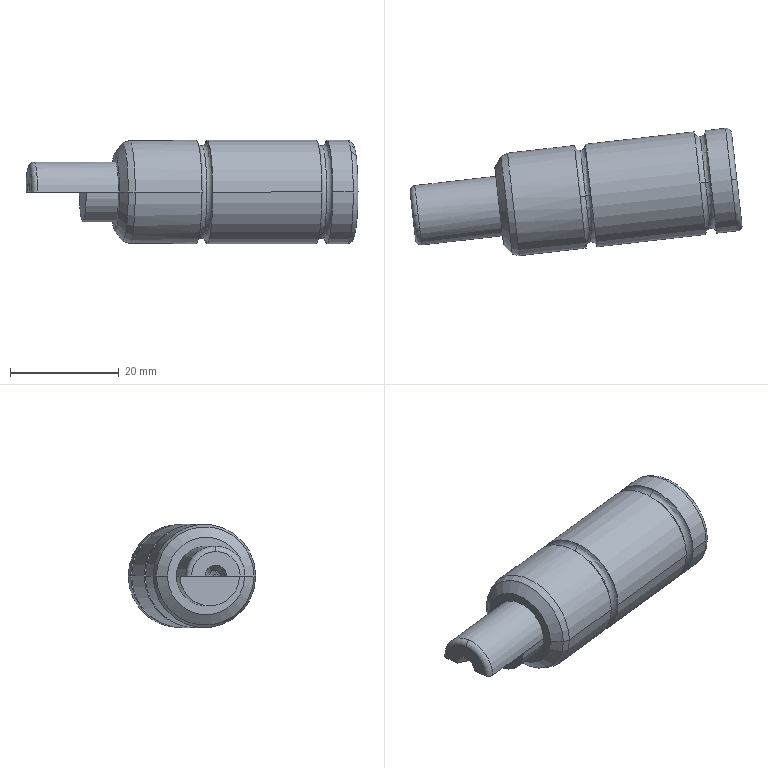Part | NX | features XQ 2 | 1 solid | 174 faces | box 61.099 x 23.455 x 19 mm | volume 13085 mm3 | plane 115 | spline 30 | torus 12 | cylinder 11 | cone 6 | commonest cylinder face diameters 19 x6 4.9 x2 11 x2 2 x1